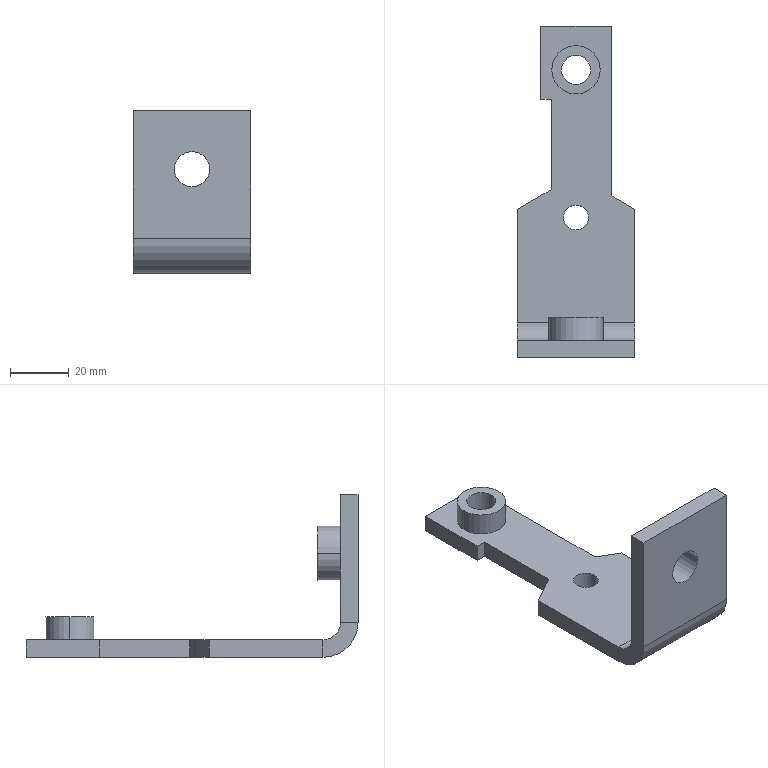Part | STEP file | 64586840 | 1 solid | 34 faces | box 40 x 113.5 x 55.6 mm | volume 32574 mm3 | plane 22 | cylinder 12 | commonest cylinder face diameters 12 x3 8.5 x2 10 x2 16.55 x2 18.5 x2 24 x1